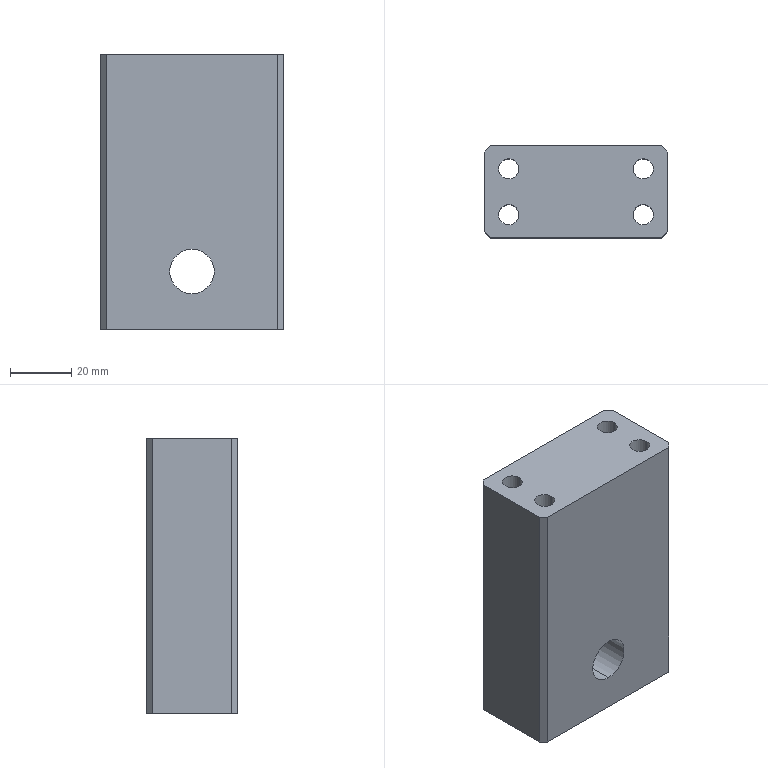Part | SolidWorks | features HoleWzd 2, Chamfer 1, Extrusion 1 | 1 solid | 32 faces | box 60 x 30 x 90 mm | volume 136711 mm3 | cylinder 18 | plane 14 | commonest cylinder face diameters 6.6 x8 11 x8 14.5 x2
STEP:
#1=CARTESIAN_POINT('',(-16.5,-7.5,30.));
#2=VERTEX_POINT('',#1);
#3=CARTESIAN_POINT('',(-27.5,-7.5,30.));
#4=VERTEX_POINT('',#3);
#5=CARTESIAN_POINT('',(-22.,-7.5,30.));
#6=DIRECTION('',(0.,0.,-1.));
#7=DIRECTION('',(-1.,0.,0.));
#8=AXIS2_PLACEMENT_3D('',#5,#6,#7);
#9=CIRCLE('',#8,5.5);
#10=EDGE_CURVE('',#2,#4,#9,.T.);
#11=ORIENTED_EDGE('',*,*,#10,.F.);
#12=CARTESIAN_POINT('',(-16.5,-7.5,0.));
#13=VERTEX_POINT('',#12);
#14=CARTESIAN_POINT('',(-16.5,-7.5,0.));
#15=DIRECTION('',(0.,0.,-1.));
#16=VECTOR('',#15,1000.);
#17=LINE('',#14,#16);
#18=EDGE_CURVE('',#2,#13,#17,.T.);
#19=ORIENTED_EDGE('',*,*,#18,.T.);
#20=CARTESIAN_POINT('',(-27.5,-7.5,0.));
#21=VERTEX_POINT('',#20);
#22=CARTESIAN_POINT('',(-22.,-7.5,0.));
#23=DIRECTION('',(0.,0.,-1.));
#24=DIRECTION('',(-1.,0.,0.));
#25=AXIS2_PLACEMENT_3D('',#22,#23,#24);
#26=CIRCLE('',#25,5.5);
#27=EDGE_CURVE('',#13,#21,#26,.T.);
#28=ORIENTED_EDGE('',*,*,#27,.T.);
#29=CARTESIAN_POINT('',(-27.5,-7.5,0.));
#30=DIRECTION('',(0.,0.,-1.));
#31=VECTOR('',#30,1000.);
#32=LINE('',#29,#31);
#33=EDGE_CURVE('',#4,#21,#32,.T.);
#34=ORIENTED_EDGE('',*,*,#33,.F.);
#35=EDGE_LOOP('',(#11,#19,#28,#34));
#36=FACE_OUTER_BOUND('',#35,.T.);
#37=CARTESIAN_POINT('',(-22.,-7.5,0.));
#38=DIRECTION('',(0.,0.,-1.));
#39=DIRECTION('',(-1.,0.,0.));
#40=AXIS2_PLACEMENT_3D('',#37,#38,#39);
#41=CYLINDRICAL_SURFACE('',#40,5.5);
#42=ADVANCED_FACE('',(#36),#41,.F.);
#43=CARTESIAN_POINT('',(-18.7,-7.5,90.));
#44=VERTEX_POINT('',#43);
#45=CARTESIAN_POINT('',(-25.3,-7.5,90.));
#46=VERTEX_POINT('',#45);
#47=CARTESIAN_POINT('',(-22.,-7.5,90.));
#48=DIRECTION('',(0.,0.,-1.));
#49=DIRECTION('',(-1.,0.,0.));
#50=AXIS2_PLACEMENT_3D('',#47,#48,#49);
#51=CIRCLE('',#50,3.3);
#52=EDGE_CURVE('',#44,#46,#51,.T.);
#53=ORIENTED_EDGE('',*,*,#52,.F.);
#54=CARTESIAN_POINT('',(-18.7,-7.5,30.));
#55=VERTEX_POINT('',#54);
#56=CARTESIAN_POINT('',(-18.7,-7.5,0.));
#57=DIRECTION('',(0.,0.,-1.));
#58=VECTOR('',#57,1000.);
#59=LINE('',#56,#58);
#60=EDGE_CURVE('',#44,#55,#59,.T.);
#61=ORIENTED_EDGE('',*,*,#60,.T.);
#62=CARTESIAN_POINT('',(-25.3,-7.5,30.));
#63=VERTEX_POINT('',#62);
#64=CARTESIAN_POINT('',(-22.,-7.5,30.));
#65=DIRECTION('',(0.,0.,-1.));
#66=DIRECTION('',(-1.,0.,0.));
#67=AXIS2_PLACEMENT_3D('',#64,#65,#66);
#68=CIRCLE('',#67,3.3);
#69=EDGE_CURVE('',#55,#63,#68,.T.);
#70=ORIENTED_EDGE('',*,*,#69,.T.);
#71=CARTESIAN_POINT('',(-25.3,-7.5,0.));
#72=DIRECTION('',(0.,0.,-1.));
#73=VECTOR('',#72,1000.);
#74=LINE('',#71,#73);
#75=EDGE_CURVE('',#46,#63,#74,.T.);
#76=ORIENTED_EDGE('',*,*,#75,.F.);
#77=EDGE_LOOP('',(#53,#61,#70,#76));
#78=FACE_OUTER_BOUND('',#77,.T.);
#79=CARTESIAN_POINT('',(-22.,-7.5,0.));
#80=DIRECTION('',(0.,0.,-1.));
#81=DIRECTION('',(-1.,0.,0.));
#82=AXIS2_PLACEMENT_3D('',#79,#80,#81);
#83=CYLINDRICAL_SURFACE('',#82,3.3);
#84=ADVANCED_FACE('',(#78),#83,.F.);
#85=CARTESIAN_POINT('',(-16.5,7.5,30.));
#86=VERTEX_POINT('',#85);
#87=CARTESIAN_POINT('',(-27.5,7.5,30.));
#88=VERTEX_POINT('',#87);
#89=CARTESIAN_POINT('',(-22.,7.5,30.));
#90=DIRECTION('',(0.,0.,-1.));
#91=DIRECTION('',(-1.,0.,0.));
#92=AXIS2_PLACEMENT_3D('',#89,#90,#91);
#93=CIRCLE('',#92,5.5);
#94=EDGE_CURVE('',#86,#88,#93,.T.);
#95=ORIENTED_EDGE('',*,*,#94,.F.);
#96=CARTESIAN_POINT('',(-16.5,7.5,0.));
#97=VERTEX_POINT('',#96);
#98=CARTESIAN_POINT('',(-16.5,7.5,0.));
#99=DIRECTION('',(0.,0.,-1.));
#100=VECTOR('',#99,1000.);
#101=LINE('',#98,#100);
#102=EDGE_CURVE('',#86,#97,#101,.T.);
#103=ORIENTED_EDGE('',*,*,#102,.T.);
#104=CARTESIAN_POINT('',(-27.5,7.5,0.));
#105=VERTEX_POINT('',#104);
#106=CARTESIAN_POINT('',(-22.,7.5,0.));
#107=DIRECTION('',(0.,0.,-1.));
#108=DIRECTION('',(-1.,0.,0.));
#109=AXIS2_PLACEMENT_3D('',#106,#107,#108);
#110=CIRCLE('',#109,5.5);
#111=EDGE_CURVE('',#97,#105,#110,.T.);
#112=ORIENTED_EDGE('',*,*,#111,.T.);
#113=CARTESIAN_POINT('',(-27.5,7.5,0.));
#114=DIRECTION('',(0.,0.,-1.));
#115=VECTOR('',#114,1000.);
#116=LINE('',#113,#115);
#117=EDGE_CURVE('',#88,#105,#116,.T.);
#118=ORIENTED_EDGE('',*,*,#117,.F.);
#119=EDGE_LOOP('',(#95,#103,#112,#118));
#120=FACE_OUTER_BOUND('',#119,.T.);
#121=CARTESIAN_POINT('',(-22.,7.5,0.));
#122=DIRECTION('',(0.,0.,-1.));
#123=DIRECTION('',(-1.,0.,0.));
#124=AXIS2_PLACEMENT_3D('',#121,#122,#123);
#125=CYLINDRICAL_SURFACE('',#124,5.5);
#126=ADVANCED_FACE('',(#120),#125,.F.);
#127=CARTESIAN_POINT('',(-18.7,7.5,90.));
#128=VERTEX_POINT('',#127);
#129=CARTESIAN_POINT('',(-25.3,7.5,90.));
#130=VERTEX_POINT('',#129);
#131=CARTESIAN_POINT('',(-22.,7.5,90.));
#132=DIRECTION('',(0.,0.,-1.));
#133=DIRECTION('',(-1.,0.,0.));
#134=AXIS2_PLACEMENT_3D('',#131,#132,#133);
#135=CIRCLE('',#134,3.3);
#136=EDGE_CURVE('',#128,#130,#135,.T.);
#137=ORIENTED_EDGE('',*,*,#136,.F.);
#138=CARTESIAN_POINT('',(-18.7,7.5,30.));
#139=VERTEX_POINT('',#138);
#140=CARTESIAN_POINT('',(-18.7,7.5,0.));
#141=DIRECTION('',(0.,0.,-1.));
#142=VECTOR('',#141,1000.);
#143=LINE('',#140,#142);
#144=EDGE_CURVE('',#128,#139,#143,.T.);
#145=ORIENTED_EDGE('',*,*,#144,.T.);
#146=CARTESIAN_POINT('',(-25.3,7.5,30.));
#147=VERTEX_POINT('',#146);
#148=CARTESIAN_POINT('',(-22.,7.5,30.));
#149=DIRECTION('',(0.,0.,-1.));
#150=DIRECTION('',(-1.,0.,0.));
#151=AXIS2_PLACEMENT_3D('',#148,#149,#150);
#152=CIRCLE('',#151,3.3);
#153=EDGE_CURVE('',#139,#147,#152,.T.);
#154=ORIENTED_EDGE('',*,*,#153,.T.);
#155=CARTESIAN_POINT('',(-25.3,7.5,0.));
#156=DIRECTION('',(0.,0.,-1.));
#157=VECTOR('',#156,1000.);
#158=LINE('',#155,#157);
#159=EDGE_CURVE('',#130,#147,#158,.T.);
#160=ORIENTED_EDGE('',*,*,#159,.F.);
#161=EDGE_LOOP('',(#137,#145,#154,#160));
#162=FACE_OUTER_BOUND('',#161,.T.);
#163=CARTESIAN_POINT('',(-22.,7.5,0.));
#164=DIRECTION('',(0.,0.,-1.));
#165=DIRECTION('',(-1.,0.,0.));
#166=AXIS2_PLACEMENT_3D('',#163,#164,#165);
#167=CYLINDRICAL_SURFACE('',#166,3.3);
#168=ADVANCED_FACE('',(#162),#167,.F.);
#169=CARTESIAN_POINT('',(27.5,7.5,30.));
#170=VERTEX_POINT('',#169);
#171=CARTESIAN_POINT('',(16.5,7.5,30.));
#172=VERTEX_POINT('',#171);
#173=CARTESIAN_POINT('',(22.,7.5,30.));
#174=DIRECTION('',(0.,0.,-1.));
#175=DIRECTION('',(-1.,0.,0.));
#176=AXIS2_PLACEMENT_3D('',#173,#174,#175);
#177=CIRCLE('',#176,5.5);
#178=EDGE_CURVE('',#170,#172,#177,.T.);
#179=ORIENTED_EDGE('',*,*,#178,.F.);
#180=CARTESIAN_POINT('',(27.5,7.5,0.));
#181=VERTEX_POINT('',#180);
#182=CARTESIAN_POINT('',(27.5,7.5,0.));
#183=DIRECTION('',(0.,0.,-1.));
#184=VECTOR('',#183,1000.);
#185=LINE('',#182,#184);
#186=EDGE_CURVE('',#170,#181,#185,.T.);
#187=ORIENTED_EDGE('',*,*,#186,.T.);
#188=CARTESIAN_POINT('',(16.5,7.5,0.));
#189=VERTEX_POINT('',#188);
#190=CARTESIAN_POINT('',(22.,7.5,0.));
#191=DIRECTION('',(0.,0.,-1.));
#192=DIRECTION('',(-1.,0.,0.));
#193=AXIS2_PLACEMENT_3D('',#190,#191,#192);
#194=CIRCLE('',#193,5.5);
#195=EDGE_CURVE('',#181,#189,#194,.T.);
#196=ORIENTED_EDGE('',*,*,#195,.T.);
#197=CARTESIAN_POINT('',(16.5,7.5,0.));
#198=DIRECTION('',(0.,0.,-1.));
#199=VECTOR('',#198,1000.);
#200=LINE('',#197,#199);
#201=EDGE_CURVE('',#172,#189,#200,.T.);
#202=ORIENTED_EDGE('',*,*,#201,.F.);
#203=EDGE_LOOP('',(#179,#187,#196,#202));
#204=FACE_OUTER_BOUND('',#203,.T.);
#205=CARTESIAN_POINT('',(22.,7.5,0.));
#206=DIRECTION('',(0.,0.,-1.));
#207=DIRECTION('',(-1.,0.,0.));
#208=AXIS2_PLACEMENT_3D('',#205,#206,#207);
#209=CYLINDRICAL_SURFACE('',#208,5.5);
#210=ADVANCED_FACE('',(#204),#209,.F.);
#211=CARTESIAN_POINT('',(25.3,7.5,90.));
#212=VERTEX_POINT('',#211);
#213=CARTESIAN_POINT('',(18.7,7.5,90.));
#214=VERTEX_POINT('',#213);
#215=CARTESIAN_POINT('',(22.,7.5,90.));
#216=DIRECTION('',(0.,0.,-1.));
#217=DIRECTION('',(-1.,0.,0.));
#218=AXIS2_PLACEMENT_3D('',#215,#216,#217);
#219=CIRCLE('',#218,3.3);
#220=EDGE_CURVE('',#212,#214,#219,.T.);
#221=ORIENTED_EDGE('',*,*,#220,.F.);
#222=CARTESIAN_POINT('',(25.3,7.5,30.));
#223=VERTEX_POINT('',#222);
#224=CARTESIAN_POINT('',(25.3,7.5,0.));
#225=DIRECTION('',(0.,0.,-1.));
#226=VECTOR('',#225,1000.);
#227=LINE('',#224,#226);
#228=EDGE_CURVE('',#212,#223,#227,.T.);
#229=ORIENTED_EDGE('',*,*,#228,.T.);
#230=CARTESIAN_POINT('',(18.7,7.5,30.));
#231=VERTEX_POINT('',#230);
#232=CARTESIAN_POINT('',(22.,7.5,30.));
#233=DIRECTION('',(0.,0.,-1.));
#234=DIRECTION('',(-1.,0.,0.));
#235=AXIS2_PLACEMENT_3D('',#232,#233,#234);
#236=CIRCLE('',#235,3.3);
#237=EDGE_CURVE('',#223,#231,#236,.T.);
#238=ORIENTED_EDGE('',*,*,#237,.T.);
#239=CARTESIAN_POINT('',(18.7,7.5,0.));
#240=DIRECTION('',(0.,0.,-1.));
#241=VECTOR('',#240,1000.);
#242=LINE('',#239,#241);
#243=EDGE_CURVE('',#214,#231,#242,.T.);
#244=ORIENTED_EDGE('',*,*,#243,.F.);
#245=EDGE_LOOP('',(#221,#229,#238,#244));
#246=FACE_OUTER_BOUND('',#245,.T.);
#247=CARTESIAN_POINT('',(22.,7.5,0.));
#248=DIRECTION('',(0.,0.,-1.));
#249=DIRECTION('',(-1.,0.,0.));
#250=AXIS2_PLACEMENT_3D('',#247,#248,#249);
#251=CYLINDRICAL_SURFACE('',#250,3.3);
#252=ADVANCED_FACE('',(#246),#251,.F.);
#253=CARTESIAN_POINT('',(27.5,-7.5,30.));
#254=VERTEX_POINT('',#253);
#255=CARTESIAN_POINT('',(16.5,-7.5,30.));
#256=VERTEX_POINT('',#255);
#257=CARTESIAN_POINT('',(22.,-7.5,30.));
#258=DIRECTION('',(0.,0.,-1.));
#259=DIRECTION('',(-1.,0.,0.));
#260=AXIS2_PLACEMENT_3D('',#257,#258,#259);
#261=CIRCLE('',#260,5.5);
#262=EDGE_CURVE('',#254,#256,#261,.T.);
#263=ORIENTED_EDGE('',*,*,#262,.F.);
#264=CARTESIAN_POINT('',(27.5,-7.5,0.));
#265=VERTEX_POINT('',#264);
#266=CARTESIAN_POINT('',(27.5,-7.5,0.));
#267=DIRECTION('',(0.,0.,-1.));
#268=VECTOR('',#267,1000.);
#269=LINE('',#266,#268);
#270=EDGE_CURVE('',#254,#265,#269,.T.);
#271=ORIENTED_EDGE('',*,*,#270,.T.);
#272=CARTESIAN_POINT('',(16.5,-7.5,0.));
#273=VERTEX_POINT('',#272);
#274=CARTESIAN_POINT('',(22.,-7.5,0.));
#275=DIRECTION('',(0.,0.,-1.));
#276=DIRECTION('',(-1.,0.,0.));
#277=AXIS2_PLACEMENT_3D('',#274,#275,#276);
#278=CIRCLE('',#277,5.5);
#279=EDGE_CURVE('',#265,#273,#278,.T.);
#280=ORIENTED_EDGE('',*,*,#279,.T.);
#281=CARTESIAN_POINT('',(16.5,-7.5,0.));
#282=DIRECTION('',(0.,0.,-1.));
#283=VECTOR('',#282,1000.);
#284=LINE('',#281,#283);
#285=EDGE_CURVE('',#256,#273,#284,.T.);
#286=ORIENTED_EDGE('',*,*,#285,.F.);
#287=EDGE_LOOP('',(#263,#271,#280,#286));
#288=FACE_OUTER_BOUND('',#287,.T.);
#289=CARTESIAN_POINT('',(22.,-7.5,0.));
#290=DIRECTION('',(0.,0.,-1.));
#291=DIRECTION('',(-1.,0.,0.));
#292=AXIS2_PLACEMENT_3D('',#289,#290,#291);
#293=CYLINDRICAL_SURFACE('',#292,5.5);
#294=ADVANCED_FACE('',(#288),#293,.F.);
#295=CARTESIAN_POINT('',(25.3,-7.5,90.));
#296=VERTEX_POINT('',#295);
#297=CARTESIAN_POINT('',(18.7,-7.5,90.));
#298=VERTEX_POINT('',#297);
#299=CARTESIAN_POINT('',(22.,-7.5,90.));
#300=DIRECTION('',(0.,0.,-1.));
#301=DIRECTION('',(-1.,0.,0.));
#302=AXIS2_PLACEMENT_3D('',#299,#300,#301);
#303=CIRCLE('',#302,3.3);
#304=EDGE_CURVE('',#296,#298,#303,.T.);
#305=ORIENTED_EDGE('',*,*,#304,.F.);
#306=CARTESIAN_POINT('',(25.3,-7.5,30.));
#307=VERTEX_POINT('',#306);
#308=CARTESIAN_POINT('',(25.3,-7.5,0.));
#309=DIRECTION('',(0.,0.,-1.));
#310=VECTOR('',#309,1000.);
#311=LINE('',#308,#310);
#312=EDGE_CURVE('',#296,#307,#311,.T.);
#313=ORIENTED_EDGE('',*,*,#312,.T.);
#314=CARTESIAN_POINT('',(18.7,-7.5,30.));
#315=VERTEX_POINT('',#314);
#316=CARTESIAN_POINT('',(22.,-7.5,30.));
#317=DIRECTION('',(0.,0.,-1.));
#318=DIRECTION('',(-1.,0.,0.));
#319=AXIS2_PLACEMENT_3D('',#316,#317,#318);
#320=CIRCLE('',#319,3.3);
#321=EDGE_CURVE('',#307,#315,#320,.T.);
#322=ORIENTED_EDGE('',*,*,#321,.T.);
#323=CARTESIAN_POINT('',(18.7,-7.5,0.));
#324=DIRECTION('',(0.,0.,-1.));
#325=VECTOR('',#324,1000.);
#326=LINE('',#323,#325);
#327=EDGE_CURVE('',#298,#315,#326,.T.);
#328=ORIENTED_EDGE('',*,*,#327,.F.);
#329=EDGE_LOOP('',(#305,#313,#322,#328));
#330=FACE_OUTER_BOUND('',#329,.T.);
#331=CARTESIAN_POINT('',(22.,-7.5,0.));
#332=DIRECTION('',(0.,0.,-1.));
#333=DIRECTION('',(-1.,0.,0.));
#334=AXIS2_PLACEMENT_3D('',#331,#332,#333);
#335=CYLINDRICAL_SURFACE('',#334,3.3);
#336=ADVANCED_FACE('',(#330),#335,.F.);
#337=CARTESIAN_POINT('',(0.,15.,26.25));
#338=VERTEX_POINT('',#337);
#339=CARTESIAN_POINT('',(0.,15.,11.75));
#340=VERTEX_POINT('',#339);
#341=CARTESIAN_POINT('',(0.,15.,19.));
#342=DIRECTION('',(0.,-1.,0.));
#343=DIRECTION('',(0.,0.,-1.));
#344=AXIS2_PLACEMENT_3D('',#341,#342,#343);
#345=CIRCLE('',#344,7.25);
#346=EDGE_CURVE('',#338,#340,#345,.T.);
#347=ORIENTED_EDGE('',*,*,#346,.F.);
#348=CARTESIAN_POINT('',(0.,-15.,26.25));
#349=VERTEX_POINT('',#348);
#350=CARTESIAN_POINT('',(0.,-15.,26.25));
#351=DIRECTION('',(0.,-1.,0.));
#352=VECTOR('',#351,1000.);
#353=LINE('',#350,#352);
#354=EDGE_CURVE('',#338,#349,#353,.T.);
#355=ORIENTED_EDGE('',*,*,#354,.T.);
#356=CARTESIAN_POINT('',(0.,-15.,11.75));
#357=VERTEX_POINT('',#356);
#358=CARTESIAN_POINT('',(0.,-15.,19.));
#359=DIRECTION('',(0.,-1.,0.));
#360=DIRECTION('',(0.,0.,-1.));
#361=AXIS2_PLACEMENT_3D('',#358,#359,#360);
#362=CIRCLE('',#361,7.25);
#363=EDGE_CURVE('',#349,#357,#362,.T.);
#364=ORIENTED_EDGE('',*,*,#363,.T.);
#365=CARTESIAN_POINT('',(0.,-15.,11.75));
#366=DIRECTION('',(0.,-1.,0.));
#367=VECTOR('',#366,1000.);
#368=LINE('',#365,#367);
#369=EDGE_CURVE('',#340,#357,#368,.T.);
#370=ORIENTED_EDGE('',*,*,#369,.F.);
#371=EDGE_LOOP('',(#347,#355,#364,#370));
#372=FACE_OUTER_BOUND('',#371,.T.);
#373=CARTESIAN_POINT('',(0.,-15.,19.));
#374=DIRECTION('',(0.,-1.,0.));
#375=DIRECTION('',(0.,0.,-1.));
#376=AXIS2_PLACEMENT_3D('',#373,#374,#375);
#377=CYLINDRICAL_SURFACE('',#376,7.25);
#378=ADVANCED_FACE('',(#372),#377,.F.);
#379=CARTESIAN_POINT('',(30.,-13.,0.));
#380=VERTEX_POINT('',#379);
#381=CARTESIAN_POINT('',(30.,13.,0.));
#382=VERTEX_POINT('',#381);
#383=CARTESIAN_POINT('',(30.,15.,0.));
#384=DIRECTION('',(0.,1.,0.));
#385=VECTOR('',#384,1000.);
#386=LINE('',#383,#385);
#387=EDGE_CURVE('',#380,#382,#386,.T.);
#388=ORIENTED_EDGE('',*,*,#387,.T.);
#389=CARTESIAN_POINT('',(30.,13.,90.));
#390=VERTEX_POINT('',#389);
#391=CARTESIAN_POINT('',(30.,13.,90.));
#392=DIRECTION('',(0.,0.,1.));
#393=VECTOR('',#392,1000.);
#394=LINE('',#391,#393);
#395=EDGE_CURVE('',#382,#390,#394,.T.);
#396=ORIENTED_EDGE('',*,*,#395,.T.);
#397=CARTESIAN_POINT('',(30.,-13.,90.));
#398=VERTEX_POINT('',#397);
#399=CARTESIAN_POINT('',(30.,15.,90.));
#400=DIRECTION('',(0.,1.,0.));
#401=VECTOR('',#400,1000.);
#402=LINE('',#399,#401);
#403=EDGE_CURVE('',#398,#390,#402,.T.);
#404=ORIENTED_EDGE('',*,*,#403,.F.);
#405=CARTESIAN_POINT('',(30.,-13.,90.));
#406=DIRECTION('',(0.,0.,-1.));
#407=VECTOR('',#406,1000.);
#408=LINE('',#405,#407);
#409=EDGE_CURVE('',#398,#380,#408,.T.);
#410=ORIENTED_EDGE('',*,*,#409,.T.);
#411=EDGE_LOOP('',(#388,#396,#404,#410));
#412=FACE_OUTER_BOUND('',#411,.T.);
#413=CARTESIAN_POINT('',(30.,15.,90.));
#414=DIRECTION('',(-1.,0.,0.));
#415=DIRECTION('',(0.,-1.,0.));
#416=AXIS2_PLACEMENT_3D('',#413,#414,#415);
#417=PLANE('',#416);
#418=ADVANCED_FACE('',(#412),#417,.F.);
#419=CARTESIAN_POINT('',(0.,15.,19.));
#420=DIRECTION('',(0.,-1.,0.));
#421=DIRECTION('',(0.,0.,-1.));
#422=AXIS2_PLACEMENT_3D('',#419,#420,#421);
#423=CIRCLE('',#422,7.25);
#424=EDGE_CURVE('',#340,#338,#423,.T.);
#425=ORIENTED_EDGE('',*,*,#424,.T.);
#426=ORIENTED_EDGE('',*,*,#346,.T.);
#427=EDGE_LOOP('',(#425,#426));
#428=FACE_BOUND('',#427,.T.);
#429=CARTESIAN_POINT('',(28.,15.,0.));
#430=VERTEX_POINT('',#429);
#431=CARTESIAN_POINT('',(-28.,15.,0.));
#432=VERTEX_POINT('',#431);
#433=CARTESIAN_POINT('',(-30.,15.,0.));
#434=DIRECTION('',(-1.,0.,0.));
#435=VECTOR('',#434,1000.);
#436=LINE('',#433,#435);
#437=EDGE_CURVE('',#430,#432,#436,.T.);
#438=ORIENTED_EDGE('',*,*,#437,.T.);
#439=CARTESIAN_POINT('',(-28.,15.,90.));
#440=VERTEX_POINT('',#439);
#441=CARTESIAN_POINT('',(-28.,15.,90.));
#442=DIRECTION('',(0.,0.,1.));
#443=VECTOR('',#442,1000.);
#444=LINE('',#441,#443);
#445=EDGE_CURVE('',#432,#440,#444,.T.);
#446=ORIENTED_EDGE('',*,*,#445,.T.);
#447=CARTESIAN_POINT('',(28.,15.,90.));
#448=VERTEX_POINT('',#447);
#449=CARTESIAN_POINT('',(-30.,15.,90.));
#450=DIRECTION('',(-1.,0.,0.));
#451=VECTOR('',#450,1000.);
#452=LINE('',#449,#451);
#453=EDGE_CURVE('',#448,#440,#452,.T.);
#454=ORIENTED_EDGE('',*,*,#453,.F.);
#455=CARTESIAN_POINT('',(28.,15.,90.));
#456=DIRECTION('',(0.,0.,-1.));
#457=VECTOR('',#456,1000.);
#458=LINE('',#455,#457);
#459=EDGE_CURVE('',#448,#430,#458,.T.);
#460=ORIENTED_EDGE('',*,*,#459,.T.);
#461=EDGE_LOOP('',(#438,#446,#454,#460));
#462=FACE_OUTER_BOUND('',#461,.T.);
#463=CARTESIAN_POINT('',(-30.,15.,90.));
#464=DIRECTION('',(0.,-1.,0.));
#465=DIRECTION('',(0.,0.,-1.));
#466=AXIS2_PLACEMENT_3D('',#463,#464,#465);
#467=PLANE('',#466);
#468=ADVANCED_FACE('',(#428,#462),#467,.F.);
#469=CARTESIAN_POINT('',(-30.,13.,90.));
#470=VERTEX_POINT('',#469);
#471=CARTESIAN_POINT('',(-30.,-13.,90.));
#472=VERTEX_POINT('',#471);
#473=CARTESIAN_POINT('',(-30.,15.,90.));
#474=DIRECTION('',(0.,-1.,0.));
#475=VECTOR('',#474,1000.);
#476=LINE('',#473,#475);
#477=EDGE_CURVE('',#470,#472,#476,.T.);
#478=ORIENTED_EDGE('',*,*,#477,.F.);
#479=CARTESIAN_POINT('',(-30.,13.,0.));
#480=VERTEX_POINT('',#479);
#481=CARTESIAN_POINT('',(-30.,13.,90.));
#482=DIRECTION('',(0.,0.,-1.));
#483=VECTOR('',#482,1000.);
#484=LINE('',#481,#483);
#485=EDGE_CURVE('',#470,#480,#484,.T.);
#486=ORIENTED_EDGE('',*,*,#485,.T.);
#487=CARTESIAN_POINT('',(-30.,-13.,0.));
#488=VERTEX_POINT('',#487);
#489=CARTESIAN_POINT('',(-30.,15.,0.));
#490=DIRECTION('',(0.,-1.,0.));
#491=VECTOR('',#490,1000.);
#492=LINE('',#489,#491);
#493=EDGE_CURVE('',#480,#488,#492,.T.);
#494=ORIENTED_EDGE('',*,*,#493,.T.);
#495=CARTESIAN_POINT('',(-30.,-13.,90.));
#496=DIRECTION('',(0.,0.,1.));
#497=VECTOR('',#496,1000.);
#498=LINE('',#495,#497);
#499=EDGE_CURVE('',#488,#472,#498,.T.);
#500=ORIENTED_EDGE('',*,*,#499,.T.);
#501=EDGE_LOOP('',(#478,#486,#494,#500));
#502=FACE_OUTER_BOUND('',#501,.T.);
#503=CARTESIAN_POINT('',(-30.,15.,90.));
#504=DIRECTION('',(1.,0.,0.));
#505=DIRECTION('',(0.,1.,0.));
#506=AXIS2_PLACEMENT_3D('',#503,#504,#505);
#507=PLANE('',#506);
#508=ADVANCED_FACE('',(#502),#507,.F.);
#509=CARTESIAN_POINT('',(0.,-15.,19.));
#510=DIRECTION('',(0.,-1.,0.));
#511=DIRECTION('',(0.,0.,-1.));
#512=AXIS2_PLACEMENT_3D('',#509,#510,#511);
#513=CIRCLE('',#512,7.25);
#514=EDGE_CURVE('',#357,#349,#513,.T.);
#515=ORIENTED_EDGE('',*,*,#514,.F.);
#516=ORIENTED_EDGE('',*,*,#363,.F.);
#517=EDGE_LOOP('',(#515,#516));
#518=FACE_BOUND('',#517,.T.);
#519=CARTESIAN_POINT('',(-28.,-15.,90.));
#520=VERTEX_POINT('',#519);
#521=CARTESIAN_POINT('',(28.,-15.,90.));
#522=VERTEX_POINT('',#521);
#523=CARTESIAN_POINT('',(-30.,-15.,90.));
#524=DIRECTION('',(1.,0.,0.));
#525=VECTOR('',#524,1000.);
#526=LINE('',#523,#525);
#527=EDGE_CURVE('',#520,#522,#526,.T.);
#528=ORIENTED_EDGE('',*,*,#527,.F.);
#529=CARTESIAN_POINT('',(-28.,-15.,0.));
#530=VERTEX_POINT('',#529);
#531=CARTESIAN_POINT('',(-28.,-15.,90.));
#532=DIRECTION('',(0.,0.,-1.));
#533=VECTOR('',#532,1000.);
#534=LINE('',#531,#533);
#535=EDGE_CURVE('',#520,#530,#534,.T.);
#536=ORIENTED_EDGE('',*,*,#535,.T.);
#537=CARTESIAN_POINT('',(28.,-15.,0.));
#538=VERTEX_POINT('',#537);
#539=CARTESIAN_POINT('',(-30.,-15.,0.));
#540=DIRECTION('',(1.,0.,0.));
#541=VECTOR('',#540,1000.);
#542=LINE('',#539,#541);
#543=EDGE_CURVE('',#530,#538,#542,.T.);
#544=ORIENTED_EDGE('',*,*,#543,.T.);
#545=CARTESIAN_POINT('',(28.,-15.,90.));
#546=DIRECTION('',(0.,0.,1.));
#547=VECTOR('',#546,1000.);
#548=LINE('',#545,#547);
#549=EDGE_CURVE('',#538,#522,#548,.T.);
#550=ORIENTED_EDGE('',*,*,#549,.T.);
#551=EDGE_LOOP('',(#528,#536,#544,#550));
#552=FACE_OUTER_BOUND('',#551,.T.);
#553=CARTESIAN_POINT('',(-30.,-15.,90.));
#554=DIRECTION('',(0.,1.,0.));
#555=DIRECTION('',(0.,0.,1.));
#556=AXIS2_PLACEMENT_3D('',#553,#554,#555);
#557=PLANE('',#556);
#558=ADVANCED_FACE('',(#518,#552),#557,.F.);
#559=CARTESIAN_POINT('',(-22.,-7.5,90.));
#560=DIRECTION('',(0.,0.,-1.));
#561=DIRECTION('',(-1.,0.,0.));
#562=AXIS2_PLACEMENT_3D('',#559,#560,#561);
#563=CIRCLE('',#562,3.3);
#564=EDGE_CURVE('',#46,#44,#563,.T.);
#565=ORIENTED_EDGE('',*,*,#564,.T.);
#566=ORIENTED_EDGE('',*,*,#52,.T.);
#567=EDGE_LOOP('',(#565,#566));
#568=FACE_BOUND('',#567,.T.);
#569=CARTESIAN_POINT('',(-22.,7.5,90.));
#570=DIRECTION('',(0.,0.,-1.));
#571=DIRECTION('',(-1.,0.,0.));
#572=AXIS2_PLACEMENT_3D('',#569,#570,#571);
#573=CIRCLE('',#572,3.3);
#574=EDGE_CURVE('',#130,#128,#573,.T.);
#575=ORIENTED_EDGE('',*,*,#574,.T.);
#576=ORIENTED_EDGE('',*,*,#136,.T.);
#577=EDGE_LOOP('',(#575,#576));
#578=FACE_BOUND('',#577,.T.);
#579=CARTESIAN_POINT('',(22.,7.5,90.));
#580=DIRECTION('',(0.,0.,-1.));
#581=DIRECTION('',(-1.,0.,0.));
#582=AXIS2_PLACEMENT_3D('',#579,#580,#581);
#583=CIRCLE('',#582,3.3);
#584=EDGE_CURVE('',#214,#212,#583,.T.);
#585=ORIENTED_EDGE('',*,*,#584,.T.);
#586=ORIENTED_EDGE('',*,*,#220,.T.);
#587=EDGE_LOOP('',(#585,#586));
#588=FACE_BOUND('',#587,.T.);
#589=CARTESIAN_POINT('',(22.,-7.5,90.));
#590=DIRECTION('',(0.,0.,-1.));
#591=DIRECTION('',(-1.,0.,0.));
#592=AXIS2_PLACEMENT_3D('',#589,#590,#591);
#593=CIRCLE('',#592,3.3);
#594=EDGE_CURVE('',#298,#296,#593,.T.);
#595=ORIENTED_EDGE('',*,*,#594,.T.);
#596=ORIENTED_EDGE('',*,*,#304,.T.);
#597=EDGE_LOOP('',(#595,#596));
#598=FACE_BOUND('',#597,.T.);
#599=ORIENTED_EDGE('',*,*,#453,.T.);
#600=CARTESIAN_POINT('',(-21.5,21.5,90.));
#601=DIRECTION('',(-0.7071,-0.7071,0.));
#602=VECTOR('',#601,1000.);
#603=LINE('',#600,#602);
#604=EDGE_CURVE('',#440,#470,#603,.T.);
#605=ORIENTED_EDGE('',*,*,#604,.T.);
#606=ORIENTED_EDGE('',*,*,#477,.T.);
#607=CARTESIAN_POINT('',(-21.5,-21.5,90.));
#608=DIRECTION('',(0.7071,-0.7071,0.));
#609=VECTOR('',#608,1000.);
#610=LINE('',#607,#609);
#611=EDGE_CURVE('',#472,#520,#610,.T.);
#612=ORIENTED_EDGE('',*,*,#611,.T.);
#613=ORIENTED_EDGE('',*,*,#527,.T.);
#614=CARTESIAN_POINT('',(21.5,-21.5,90.));
#615=DIRECTION('',(0.7071,0.7071,0.));
#616=VECTOR('',#615,1000.);
#617=LINE('',#614,#616);
#618=EDGE_CURVE('',#522,#398,#617,.T.);
#619=ORIENTED_EDGE('',*,*,#618,.T.);
#620=ORIENTED_EDGE('',*,*,#403,.T.);
#621=CARTESIAN_POINT('',(21.5,21.5,90.));
#622=DIRECTION('',(-0.7071,0.7071,0.));
#623=VECTOR('',#622,1000.);
#624=LINE('',#621,#623);
#625=EDGE_CURVE('',#390,#448,#624,.T.);
#626=ORIENTED_EDGE('',*,*,#625,.T.);
#627=EDGE_LOOP('',(#599,#605,#606,#612,#613,#619,#620,#626));
#628=FACE_OUTER_BOUND('',#627,.T.);
#629=CARTESIAN_POINT('',(0.,0.,90.));
#630=DIRECTION('',(0.,0.,1.));
#631=DIRECTION('',(1.,0.,0.));
#632=AXIS2_PLACEMENT_3D('',#629,#630,#631);
#633=PLANE('',#632);
#634=ADVANCED_FACE('',(#568,#578,#588,#598,#628),#633,.T.);
#635=CARTESIAN_POINT('',(-22.,-7.5,0.));
#636=DIRECTION('',(0.,0.,-1.));
#637=DIRECTION('',(-1.,0.,0.));
#638=AXIS2_PLACEMENT_3D('',#635,#636,#637);
#639=CIRCLE('',#638,5.5);
#640=EDGE_CURVE('',#21,#13,#639,.T.);
#641=ORIENTED_EDGE('',*,*,#640,.F.);
#642=ORIENTED_EDGE('',*,*,#27,.F.);
#643=EDGE_LOOP('',(#641,#642));
#644=FACE_BOUND('',#643,.T.);
#645=CARTESIAN_POINT('',(-22.,7.5,0.));
#646=DIRECTION('',(0.,0.,-1.));
#647=DIRECTION('',(-1.,0.,0.));
#648=AXIS2_PLACEMENT_3D('',#645,#646,#647);
#649=CIRCLE('',#648,5.5);
#650=EDGE_CURVE('',#105,#97,#649,.T.);
#651=ORIENTED_EDGE('',*,*,#650,.F.);
#652=ORIENTED_EDGE('',*,*,#111,.F.);
#653=EDGE_LOOP('',(#651,#652));
#654=FACE_BOUND('',#653,.T.);
#655=CARTESIAN_POINT('',(22.,7.5,0.));
#656=DIRECTION('',(0.,0.,-1.));
#657=DIRECTION('',(-1.,0.,0.));
#658=AXIS2_PLACEMENT_3D('',#655,#656,#657);
#659=CIRCLE('',#658,5.5);
#660=EDGE_CURVE('',#189,#181,#659,.T.);
#661=ORIENTED_EDGE('',*,*,#660,.F.);
#662=ORIENTED_EDGE('',*,*,#195,.F.);
#663=EDGE_LOOP('',(#661,#662));
#664=FACE_BOUND('',#663,.T.);
#665=CARTESIAN_POINT('',(22.,-7.5,0.));
#666=DIRECTION('',(0.,0.,-1.));
#667=DIRECTION('',(-1.,0.,0.));
#668=AXIS2_PLACEMENT_3D('',#665,#666,#667);
#669=CIRCLE('',#668,5.5);
#670=EDGE_CURVE('',#273,#265,#669,.T.);
#671=ORIENTED_EDGE('',*,*,#670,.F.);
#672=ORIENTED_EDGE('',*,*,#279,.F.);
#673=EDGE_LOOP('',(#671,#672));
#674=FACE_BOUND('',#673,.T.);
#675=ORIENTED_EDGE('',*,*,#493,.F.);
#676=CARTESIAN_POINT('',(-30.,13.,0.));
#677=DIRECTION('',(0.7071,0.7071,0.));
#678=VECTOR('',#677,1000.);
#679=LINE('',#676,#678);
#680=EDGE_CURVE('',#480,#432,#679,.T.);
#681=ORIENTED_EDGE('',*,*,#680,.T.);
#682=ORIENTED_EDGE('',*,*,#437,.F.);
#683=CARTESIAN_POINT('',(28.,15.,0.));
#684=DIRECTION('',(0.7071,-0.7071,0.));
#685=VECTOR('',#684,1000.);
#686=LINE('',#683,#685);
#687=EDGE_CURVE('',#430,#382,#686,.T.);
#688=ORIENTED_EDGE('',*,*,#687,.T.);
#689=ORIENTED_EDGE('',*,*,#387,.F.);
#690=CARTESIAN_POINT('',(30.,-13.,0.));
#691=DIRECTION('',(-0.7071,-0.7071,0.));
#692=VECTOR('',#691,1000.);
#693=LINE('',#690,#692);
#694=EDGE_CURVE('',#380,#538,#693,.T.);
#695=ORIENTED_EDGE('',*,*,#694,.T.);
#696=ORIENTED_EDGE('',*,*,#543,.F.);
#697=CARTESIAN_POINT('',(-28.,-15.,0.));
#698=DIRECTION('',(-0.7071,0.7071,0.));
#699=VECTOR('',#698,1000.);
#700=LINE('',#697,#699);
#701=EDGE_CURVE('',#530,#488,#700,.T.);
#702=ORIENTED_EDGE('',*,*,#701,.T.);
#703=EDGE_LOOP('',(#675,#681,#682,#688,#689,#695,#696,#702));
#704=FACE_OUTER_BOUND('',#703,.T.);
#705=CARTESIAN_POINT('',(0.,0.,0.));
#706=DIRECTION('',(0.,0.,1.));
#707=DIRECTION('',(1.,0.,0.));
#708=AXIS2_PLACEMENT_3D('',#705,#706,#707);
#709=PLANE('',#708);
#710=ADVANCED_FACE('',(#644,#654,#664,#674,#704),#709,.F.);
#711=ORIENTED_EDGE('',*,*,#354,.F.);
#712=ORIENTED_EDGE('',*,*,#424,.F.);
#713=ORIENTED_EDGE('',*,*,#369,.T.);
#714=ORIENTED_EDGE('',*,*,#514,.T.);
#715=EDGE_LOOP('',(#711,#712,#713,#714));
#716=FACE_OUTER_BOUND('',#715,.T.);
#717=CARTESIAN_POINT('',(0.,-15.,19.));
#718=DIRECTION('',(0.,-1.,0.));
#719=DIRECTION('',(0.,0.,-1.));
#720=AXIS2_PLACEMENT_3D('',#717,#718,#719);
#721=CYLINDRICAL_SURFACE('',#720,7.25);
#722=ADVANCED_FACE('',(#716),#721,.F.);
#723=ORIENTED_EDGE('',*,*,#312,.F.);
#724=ORIENTED_EDGE('',*,*,#594,.F.);
#725=ORIENTED_EDGE('',*,*,#327,.T.);
#726=CARTESIAN_POINT('',(22.,-7.5,30.));
#727=DIRECTION('',(0.,0.,-1.));
#728=DIRECTION('',(-1.,0.,0.));
#729=AXIS2_PLACEMENT_3D('',#726,#727,#728);
#730=CIRCLE('',#729,3.3);
#731=EDGE_CURVE('',#315,#307,#730,.T.);
#732=ORIENTED_EDGE('',*,*,#731,.T.);
#733=EDGE_LOOP('',(#723,#724,#725,#732));
#734=FACE_OUTER_BOUND('',#733,.T.);
#735=CARTESIAN_POINT('',(22.,-7.5,0.));
#736=DIRECTION('',(0.,0.,-1.));
#737=DIRECTION('',(-1.,0.,0.));
#738=AXIS2_PLACEMENT_3D('',#735,#736,#737);
#739=CYLINDRICAL_SURFACE('',#738,3.3);
#740=ADVANCED_FACE('',(#734),#739,.F.);
#741=ORIENTED_EDGE('',*,*,#731,.F.);
#742=ORIENTED_EDGE('',*,*,#321,.F.);
#743=EDGE_LOOP('',(#741,#742));
#744=FACE_BOUND('',#743,.T.);
#745=CARTESIAN_POINT('',(22.,-7.5,30.));
#746=DIRECTION('',(0.,0.,-1.));
#747=DIRECTION('',(-1.,0.,0.));
#748=AXIS2_PLACEMENT_3D('',#745,#746,#747);
#749=CIRCLE('',#748,5.5);
#750=EDGE_CURVE('',#256,#254,#749,.T.);
#751=ORIENTED_EDGE('',*,*,#750,.T.);
#752=ORIENTED_EDGE('',*,*,#262,.T.);
#753=EDGE_LOOP('',(#751,#752));
#754=FACE_OUTER_BOUND('',#753,.T.);
#755=CARTESIAN_POINT('',(25.3,-7.5,30.));
#756=DIRECTION('',(0.,0.,1.));
#757=DIRECTION('',(1.,0.,0.));
#758=AXIS2_PLACEMENT_3D('',#755,#756,#757);
#759=PLANE('',#758);
#760=ADVANCED_FACE('',(#744,#754),#759,.F.);
#761=ORIENTED_EDGE('',*,*,#270,.F.);
#762=ORIENTED_EDGE('',*,*,#750,.F.);
#763=ORIENTED_EDGE('',*,*,#285,.T.);
#764=ORIENTED_EDGE('',*,*,#670,.T.);
#765=EDGE_LOOP('',(#761,#762,#763,#764));
#766=FACE_OUTER_BOUND('',#765,.T.);
#767=CARTESIAN_POINT('',(22.,-7.5,0.));
#768=DIRECTION('',(0.,0.,-1.));
#769=DIRECTION('',(-1.,0.,0.));
#770=AXIS2_PLACEMENT_3D('',#767,#768,#769);
#771=CYLINDRICAL_SURFACE('',#770,5.5);
#772=ADVANCED_FACE('',(#766),#771,.F.);
#773=ORIENTED_EDGE('',*,*,#228,.F.);
#774=ORIENTED_EDGE('',*,*,#584,.F.);
#775=ORIENTED_EDGE('',*,*,#243,.T.);
#776=CARTESIAN_POINT('',(22.,7.5,30.));
#777=DIRECTION('',(0.,0.,-1.));
#778=DIRECTION('',(-1.,0.,0.));
#779=AXIS2_PLACEMENT_3D('',#776,#777,#778);
#780=CIRCLE('',#779,3.3);
#781=EDGE_CURVE('',#231,#223,#780,.T.);
#782=ORIENTED_EDGE('',*,*,#781,.T.);
#783=EDGE_LOOP('',(#773,#774,#775,#782));
#784=FACE_OUTER_BOUND('',#783,.T.);
#785=CARTESIAN_POINT('',(22.,7.5,0.));
#786=DIRECTION('',(0.,0.,-1.));
#787=DIRECTION('',(-1.,0.,0.));
#788=AXIS2_PLACEMENT_3D('',#785,#786,#787);
#789=CYLINDRICAL_SURFACE('',#788,3.3);
#790=ADVANCED_FACE('',(#784),#789,.F.);
#791=ORIENTED_EDGE('',*,*,#781,.F.);
#792=ORIENTED_EDGE('',*,*,#237,.F.);
#793=EDGE_LOOP('',(#791,#792));
#794=FACE_BOUND('',#793,.T.);
#795=CARTESIAN_POINT('',(22.,7.5,30.));
#796=DIRECTION('',(0.,0.,-1.));
#797=DIRECTION('',(-1.,0.,0.));
#798=AXIS2_PLACEMENT_3D('',#795,#796,#797);
#799=CIRCLE('',#798,5.5);
#800=EDGE_CURVE('',#172,#170,#799,.T.);
#801=ORIENTED_EDGE('',*,*,#800,.T.);
#802=ORIENTED_EDGE('',*,*,#178,.T.);
#803=EDGE_LOOP('',(#801,#802));
#804=FACE_OUTER_BOUND('',#803,.T.);
#805=CARTESIAN_POINT('',(25.3,7.5,30.));
#806=DIRECTION('',(0.,0.,1.));
#807=DIRECTION('',(1.,0.,0.));
#808=AXIS2_PLACEMENT_3D('',#805,#806,#807);
#809=PLANE('',#808);
#810=ADVANCED_FACE('',(#794,#804),#809,.F.);
#811=ORIENTED_EDGE('',*,*,#186,.F.);
#812=ORIENTED_EDGE('',*,*,#800,.F.);
#813=ORIENTED_EDGE('',*,*,#201,.T.);
#814=ORIENTED_EDGE('',*,*,#660,.T.);
#815=EDGE_LOOP('',(#811,#812,#813,#814));
#816=FACE_OUTER_BOUND('',#815,.T.);
#817=CARTESIAN_POINT('',(22.,7.5,0.));
#818=DIRECTION('',(0.,0.,-1.));
#819=DIRECTION('',(-1.,0.,0.));
#820=AXIS2_PLACEMENT_3D('',#817,#818,#819);
#821=CYLINDRICAL_SURFACE('',#820,5.5);
#822=ADVANCED_FACE('',(#816),#821,.F.);
#823=ORIENTED_EDGE('',*,*,#144,.F.);
#824=ORIENTED_EDGE('',*,*,#574,.F.);
#825=ORIENTED_EDGE('',*,*,#159,.T.);
#826=CARTESIAN_POINT('',(-22.,7.5,30.));
#827=DIRECTION('',(0.,0.,-1.));
#828=DIRECTION('',(-1.,0.,0.));
#829=AXIS2_PLACEMENT_3D('',#826,#827,#828);
#830=CIRCLE('',#829,3.3);
#831=EDGE_CURVE('',#147,#139,#830,.T.);
#832=ORIENTED_EDGE('',*,*,#831,.T.);
#833=EDGE_LOOP('',(#823,#824,#825,#832));
#834=FACE_OUTER_BOUND('',#833,.T.);
#835=CARTESIAN_POINT('',(-22.,7.5,0.));
#836=DIRECTION('',(0.,0.,-1.));
#837=DIRECTION('',(-1.,0.,0.));
#838=AXIS2_PLACEMENT_3D('',#835,#836,#837);
#839=CYLINDRICAL_SURFACE('',#838,3.3);
#840=ADVANCED_FACE('',(#834),#839,.F.);
#841=ORIENTED_EDGE('',*,*,#831,.F.);
#842=ORIENTED_EDGE('',*,*,#153,.F.);
#843=EDGE_LOOP('',(#841,#842));
#844=FACE_BOUND('',#843,.T.);
#845=CARTESIAN_POINT('',(-22.,7.5,30.));
#846=DIRECTION('',(0.,0.,-1.));
#847=DIRECTION('',(-1.,0.,0.));
#848=AXIS2_PLACEMENT_3D('',#845,#846,#847);
#849=CIRCLE('',#848,5.5);
#850=EDGE_CURVE('',#88,#86,#849,.T.);
#851=ORIENTED_EDGE('',*,*,#850,.T.);
#852=ORIENTED_EDGE('',*,*,#94,.T.);
#853=EDGE_LOOP('',(#851,#852));
#854=FACE_OUTER_BOUND('',#853,.T.);
#855=CARTESIAN_POINT('',(-18.7,7.5,30.));
#856=DIRECTION('',(0.,0.,1.));
#857=DIRECTION('',(1.,0.,0.));
#858=AXIS2_PLACEMENT_3D('',#855,#856,#857);
#859=PLANE('',#858);
#860=ADVANCED_FACE('',(#844,#854),#859,.F.);
#861=ORIENTED_EDGE('',*,*,#102,.F.);
#862=ORIENTED_EDGE('',*,*,#850,.F.);
#863=ORIENTED_EDGE('',*,*,#117,.T.);
#864=ORIENTED_EDGE('',*,*,#650,.T.);
#865=EDGE_LOOP('',(#861,#862,#863,#864));
#866=FACE_OUTER_BOUND('',#865,.T.);
#867=CARTESIAN_POINT('',(-22.,7.5,0.));
#868=DIRECTION('',(0.,0.,-1.));
#869=DIRECTION('',(-1.,0.,0.));
#870=AXIS2_PLACEMENT_3D('',#867,#868,#869);
#871=CYLINDRICAL_SURFACE('',#870,5.5);
#872=ADVANCED_FACE('',(#866),#871,.F.);
#873=ORIENTED_EDGE('',*,*,#60,.F.);
#874=ORIENTED_EDGE('',*,*,#564,.F.);
#875=ORIENTED_EDGE('',*,*,#75,.T.);
#876=CARTESIAN_POINT('',(-22.,-7.5,30.));
#877=DIRECTION('',(0.,0.,-1.));
#878=DIRECTION('',(-1.,0.,0.));
#879=AXIS2_PLACEMENT_3D('',#876,#877,#878);
#880=CIRCLE('',#879,3.3);
#881=EDGE_CURVE('',#63,#55,#880,.T.);
#882=ORIENTED_EDGE('',*,*,#881,.T.);
#883=EDGE_LOOP('',(#873,#874,#875,#882));
#884=FACE_OUTER_BOUND('',#883,.T.);
#885=CARTESIAN_POINT('',(-22.,-7.5,0.));
#886=DIRECTION('',(0.,0.,-1.));
#887=DIRECTION('',(-1.,0.,0.));
#888=AXIS2_PLACEMENT_3D('',#885,#886,#887);
#889=CYLINDRICAL_SURFACE('',#888,3.3);
#890=ADVANCED_FACE('',(#884),#889,.F.);
#891=ORIENTED_EDGE('',*,*,#881,.F.);
#892=ORIENTED_EDGE('',*,*,#69,.F.);
#893=EDGE_LOOP('',(#891,#892));
#894=FACE_BOUND('',#893,.T.);
#895=CARTESIAN_POINT('',(-22.,-7.5,30.));
#896=DIRECTION('',(0.,0.,-1.));
#897=DIRECTION('',(-1.,0.,0.));
#898=AXIS2_PLACEMENT_3D('',#895,#896,#897);
#899=CIRCLE('',#898,5.5);
#900=EDGE_CURVE('',#4,#2,#899,.T.);
#901=ORIENTED_EDGE('',*,*,#900,.T.);
#902=ORIENTED_EDGE('',*,*,#10,.T.);
#903=EDGE_LOOP('',(#901,#902));
#904=FACE_OUTER_BOUND('',#903,.T.);
#905=CARTESIAN_POINT('',(-18.7,-7.5,30.));
#906=DIRECTION('',(0.,0.,1.));
#907=DIRECTION('',(1.,0.,0.));
#908=AXIS2_PLACEMENT_3D('',#905,#906,#907);
#909=PLANE('',#908);
#910=ADVANCED_FACE('',(#894,#904),#909,.F.);
#911=ORIENTED_EDGE('',*,*,#18,.F.);
#912=ORIENTED_EDGE('',*,*,#900,.F.);
#913=ORIENTED_EDGE('',*,*,#33,.T.);
#914=ORIENTED_EDGE('',*,*,#640,.T.);
#915=EDGE_LOOP('',(#911,#912,#913,#914));
#916=FACE_OUTER_BOUND('',#915,.T.);
#917=CARTESIAN_POINT('',(-22.,-7.5,0.));
#918=DIRECTION('',(0.,0.,-1.));
#919=DIRECTION('',(-1.,0.,0.));
#920=AXIS2_PLACEMENT_3D('',#917,#918,#919);
#921=CYLINDRICAL_SURFACE('',#920,5.5);
#922=ADVANCED_FACE('',(#916),#921,.F.);
#923=ORIENTED_EDGE('',*,*,#604,.F.);
#924=ORIENTED_EDGE('',*,*,#445,.F.);
#925=ORIENTED_EDGE('',*,*,#680,.F.);
#926=ORIENTED_EDGE('',*,*,#485,.F.);
#927=EDGE_LOOP('',(#923,#924,#925,#926));
#928=FACE_OUTER_BOUND('',#927,.T.);
#929=CARTESIAN_POINT('',(-30.,13.,90.));
#930=DIRECTION('',(0.7071,-0.7071,0.));
#931=DIRECTION('',(0.,0.,-1.));
#932=AXIS2_PLACEMENT_3D('',#929,#930,#931);
#933=PLANE('',#932);
#934=ADVANCED_FACE('',(#928),#933,.F.);
#935=ORIENTED_EDGE('',*,*,#611,.F.);
#936=ORIENTED_EDGE('',*,*,#499,.F.);
#937=ORIENTED_EDGE('',*,*,#701,.F.);
#938=ORIENTED_EDGE('',*,*,#535,.F.);
#939=EDGE_LOOP('',(#935,#936,#937,#938));
#940=FACE_OUTER_BOUND('',#939,.T.);
#941=CARTESIAN_POINT('',(-28.,-15.,90.));
#942=DIRECTION('',(0.7071,0.7071,0.));
#943=DIRECTION('',(0.,0.,-1.));
#944=AXIS2_PLACEMENT_3D('',#941,#942,#943);
#945=PLANE('',#944);
#946=ADVANCED_FACE('',(#940),#945,.F.);
#947=ORIENTED_EDGE('',*,*,#625,.F.);
#948=ORIENTED_EDGE('',*,*,#395,.F.);
#949=ORIENTED_EDGE('',*,*,#687,.F.);
#950=ORIENTED_EDGE('',*,*,#459,.F.);
#951=EDGE_LOOP('',(#947,#948,#949,#950));
#952=FACE_OUTER_BOUND('',#951,.T.);
#953=CARTESIAN_POINT('',(28.,15.,90.));
#954=DIRECTION('',(-0.7071,-0.7071,0.));
#955=DIRECTION('',(0.,0.,-1.));
#956=AXIS2_PLACEMENT_3D('',#953,#954,#955);
#957=PLANE('',#956);
#958=ADVANCED_FACE('',(#952),#957,.F.);
#959=ORIENTED_EDGE('',*,*,#618,.F.);
#960=ORIENTED_EDGE('',*,*,#549,.F.);
#961=ORIENTED_EDGE('',*,*,#694,.F.);
#962=ORIENTED_EDGE('',*,*,#409,.F.);
#963=EDGE_LOOP('',(#959,#960,#961,#962));
#964=FACE_OUTER_BOUND('',#963,.T.);
#965=CARTESIAN_POINT('',(30.,-13.,90.));
#966=DIRECTION('',(-0.7071,0.7071,0.));
#967=DIRECTION('',(0.,0.,-1.));
#968=AXIS2_PLACEMENT_3D('',#965,#966,#967);
#969=PLANE('',#968);
#970=ADVANCED_FACE('',(#964),#969,.F.);
#971=CLOSED_SHELL('',(#42,#84,#126,#168,#210,#252,#294,#336,#378,#418,#468,#508,#558,#634,#710,#722,#740,#760,#772,#790,#810,#822,#840,#860,#872,#890,#910,#922,#934,#946,#958,#970));
#972=MANIFOLD_SOLID_BREP('',#971);
#973=CARTESIAN_POINT('',(0.,0.,0.));
#974=DIRECTION('',(0.,0.,1.));
#975=DIRECTION('',(1.,0.,0.));
#976=AXIS2_PLACEMENT_3D('',#973,#974,#975);
#977=(LENGTH_UNIT()NAMED_UNIT(*)SI_UNIT(.MILLI.,.METRE.));
#978=UNCERTAINTY_MEASURE_WITH_UNIT(LENGTH_MEASURE(0.00001),#977,'','');
#979=(NAMED_UNIT(*)PLANE_ANGLE_UNIT()SI_UNIT($,.RADIAN.));
#980=(NAMED_UNIT(*)SI_UNIT($,.STERADIAN.)SOLID_ANGLE_UNIT());
#981=(GEOMETRIC_REPRESENTATION_CONTEXT(3)GLOBAL_UNCERTAINTY_ASSIGNED_CONTEXT((#978))GLOBAL_UNIT_ASSIGNED_CONTEXT((#977,#979,#980))REPRESENTATION_CONTEXT('',''));
#982=ADVANCED_BREP_SHAPE_REPRESENTATION('',(#972,#976),#981);